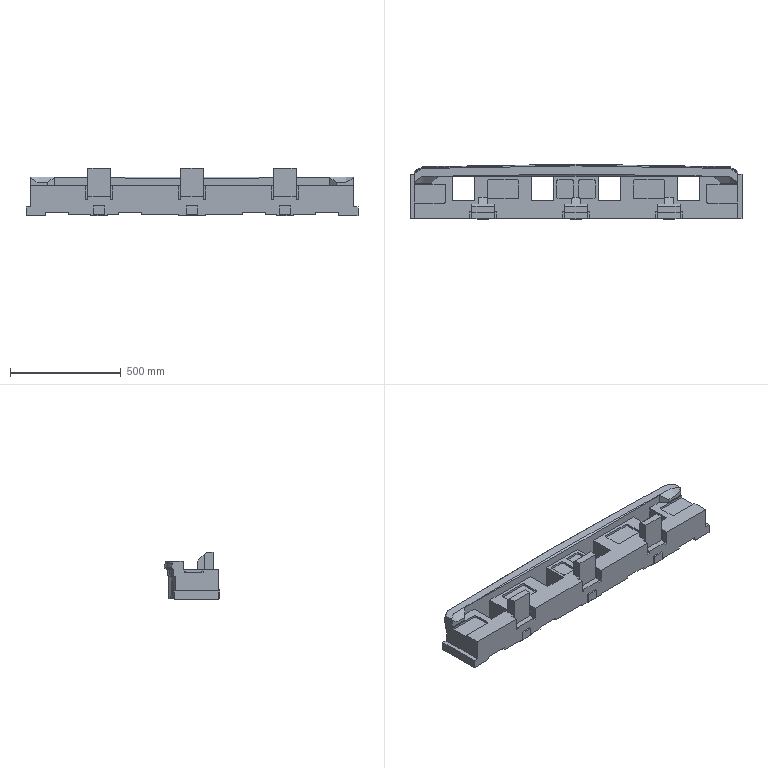Part | NX | features solid 2 | 1 solid | 357 faces | box 1500 x 249.791 x 215 mm | volume 38819856 mm3 | plane 179 | spline 142 | cylinder 36 | commonest cylinder face diameters 10 x36